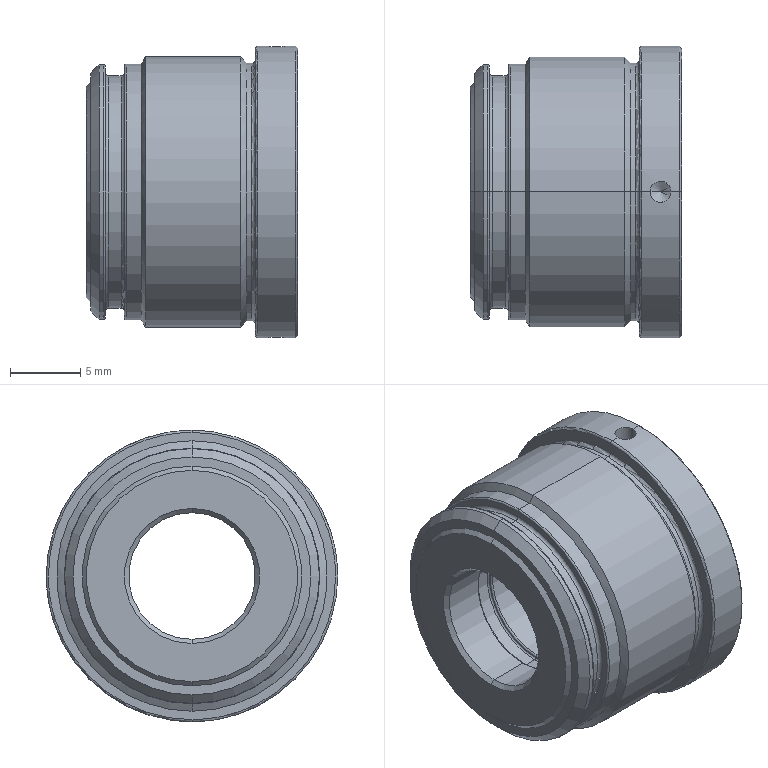Part | STEP file | 2026.6.15-Main Assembly图.sldasm-Part-222 | 1 solid | 104 faces | box 15 x 20.7 x 20.7 mm | volume 3082 mm3 | torus 38 | cylinder 34 | cone 20 | plane 12 | commonest cylinder face diameters 9 x6 1.5 x4 1.8 x4 9.6 x2 9.9 x2 11.58 x2